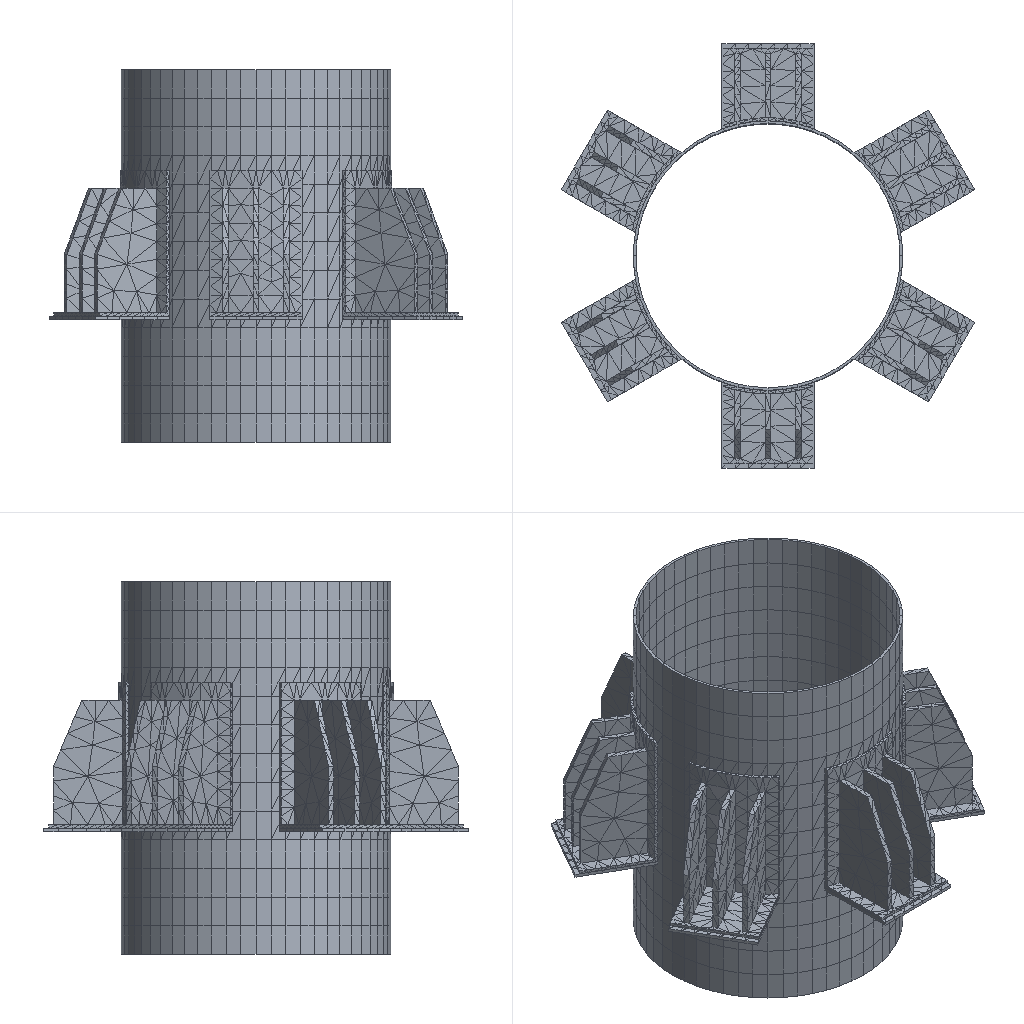Simulation study | ansys workbench
Ansys APDL input file, long lists of numbers shortened:
/batch
/config,noeldb,1     ! force off writing results to database
*get,_wallstrt,active,,time,wall
! ANSYS input file written by Workbench version 2022 R1
! File used for geometry attach:
/title,wbnew--____ (D5)
! ****** Begin Custom Load Command Snippet ******
/COM, ACT Extensions:
/COM,     LSDYNA, 2021.1
/COM,
! ****** End   Custom Load Command Snippet ******
*DIM,_wb_ProjectScratch_dir,string,248
_wb_ProjectScratch_dir(1) = ''
*DIM,_wb_SolverFiles_dir,string,248
_wb_SolverFiles_dir(1) = ''
*DIM,_wb_userfiles_dir,string,248
_wb_userfiles_dir(1) = ''
/com,--- Data in consistent NMM units. See Solving Units in the help system for more information.
/units,MPA
/nopr
/wb,file,start              !  signify a WB generated input file
/prep7
! Turn off shape checking because checks already performed inside WB mesher.
! See help system for more information.
SHPP,OFF,,NOWARN
/nolist
etcon,set             ! allow ANSYS to choose best KEYOP's for 180x elements, resets any applicable keyopt to MAPDL defaults
/com,*********** Nodes for the whole assembly ***********
nblock,3,,22077
(1i9,3e20.9e3)
        1     6.530950049E+02     2.499215719E+03     8.316464507E+02
! (20069 more lines like these left out)
-1
/wb,elem,start            !  set before creation of elements
/com,*********** Elements for Body 1 "__4^1400-589-450|__-__2" ***********
et,1,187
eblock,19,solid,,932
(19i9)
        1        1        1        1        0        0        0        0       10        0      729     5581     5723     5720     5722     7087     7383     7085     7086
! (1863 more lines like these left out)
-1
/com,*********** Elements for Body 2 "__5^1400-589-450|__-__1" ***********
et,2,186
keyo,2,2,1          ! set full integration on SOLID186
eblock,19,solid,,42
(19i9)
        2        2        2        2        0        0        0        0       20        0     6489    19376    19433    19434    19458    19377    19426    19425    19407
! (83 more lines like these left out)
-1
/com,*********** Elements for Body 3 "__5^1400-589-450|__-__1[2]" ***********
et,3,186
keyo,3,2,1          ! set full integration on SOLID186
eblock,19,solid,,42
(19i9)
        3        3        3        3        0        0        0        0       20        0     6405    18652    18709    18710    18734    18653    18702    18701    18683
! (83 more lines like these left out)
-1
/com,*********** Elements for Body 4 "__5^1400-589-450|__-__1[3]" ***********
et,4,186
keyo,4,2,1          ! set full integration on SOLID186
eblock,19,solid,,42
(19i9)
        4        4        4        4        0        0        0        0       20        0     6447    19014    19071    19072    19096    19015    19064    19063    19045
! (83 more lines like these left out)
-1
/com,*********** Elements for Body 5 "__5^1400-589-450|__-__1[4]" ***********
et,5,186
keyo,5,2,1          ! set full integration on SOLID186
eblock,19,solid,,42
(19i9)
        5        5        5        5        0        0        0        0       20        0     6531    19738    19795    19796    19820    19739    19788    19787    19769
! (83 more lines like these left out)
-1
/com,*********** Elements for Body 6 "__5^1400-589-450|__-__1[5]" ***********
et,6,186
keyo,6,2,1          ! set full integration on SOLID186
eblock,19,solid,,42
(19i9)
        6        6        6        6        0        0        0        0       20        0     6321    17928    17985    17986    18010    17929    17978    17977    17959
! (83 more lines like these left out)
-1
/com,*********** Elements for Body 7 "__5^1400-589-450|__-__1[6]" ***********
et,7,186
keyo,7,2,1          ! set full integration on SOLID186
eblock,19,solid,,42
(19i9)
        7        7        7        7        0        0        0        0       20        0     6363    18290    18347    18348    18372    18291    18340    18339    18321
! (83 more lines like these left out)
-1
/com,*********** Elements for Body 8 "__4^1400-589-450|__-__2[2]" ***********
et,8,187
eblock,19,solid,,932
(19i9)
        8        8        8        8        0        0        0        0       10        0     4457    13929    14071    14068    14070    15435    15731    15433    15434
! (1863 more lines like these left out)
-1
/com,*********** Elements for Body 9 "__4^1400-589-450|__-__2[3]" ***********
et,9,187
eblock,19,solid,,932
(19i9)
        9        9        9        9        0        0        0        0       10        0     3525    11842    11984    11981    11983    13348    13644    13346    13347
! (1863 more lines like these left out)
-1
/com,*********** Elements for Body 10 "__4^1400-589-450|__-__2[4]" ***********
et,10,187
eblock,19,solid,,932
(19i9)
       10       10       10       10        0        0        0        0       10        0     1661     7668     7810     7807     7809     9174     9470     9172     9173
! (1863 more lines like these left out)
-1
/com,*********** Elements for Body 11 "__4^1400-589-450|__-__2[5]" ***********
et,11,187
eblock,19,solid,,932
(19i9)
       11       11       11       11        0        0        0        0       10        0     5389    16016    16158    16155    16157    17522    17818    17520    17521
! (1863 more lines like these left out)
-1
/com,*********** Elements for Body 12 "__4^1400-589-450|__-__2[6]" ***********
et,12,187
eblock,19,solid,,932
(19i9)
       12       12       12       12        0        0        0        0       10        0     2593     9755     9897     9894     9896    11261    11557    11259    11260
! (1863 more lines like these left out)
-1
/com,*********** Elements for Body 13 "__3^1400-589-450|__-__1" ***********
et,13,186
keyo,13,2,1          ! set full integration on SOLID186
eblock,19,solid,,728
(19i9)
       13       13       13       13        0        0        0        0       20        0        1      113      893      843      478      437     1191      842      438
! (1455 more lines like these left out)
-1
/wb,elem,end               !  done creating elements
/com,*********** Send User Defined Coordinate System(s) ***********
csys,0
toffst,273.15,  ! Temperature offset from absolute zero
/com,*********** Set Reference Temperature ***********
tref,22.
/wb,mat,start              !  starting to send materials
/com,*********** Send Materials ***********
Temperature = 'TEMP' ! Temperature
MP,DENS,1,7.85e-09,	! tonne mm^-3
MP,ALPX,1,1.2e-05,	! C^-1
MP,C,1,434000000,	! mm^2 s^-2 C^-1
MP,KXX,1,60.5,	! tonne mm s^-3 C^-1
MP,RSVX,1,0.00017,	! ohm mm
MP,EX,1,200000,	! tonne s^-2 mm^-1
MP,NUXY,1,0.3,
MP,MURX,1,10000,
Temperature = 'TEMP' ! Temperature
MP,DENS,2,7.85e-09,	! tonne mm^-3
MP,ALPX,2,1.2e-05,	! C^-1
MP,C,2,434000000,	! mm^2 s^-2 C^-1
MP,KXX,2,60.5,	! tonne mm s^-3 C^-1
MP,RSVX,2,0.00017,	! ohm mm
MP,EX,2,200000,	! tonne s^-2 mm^-1
MP,NUXY,2,0.3,
MP,MURX,2,10000,
Temperature = 'TEMP' ! Temperature
MP,DENS,3,7.85e-09,	! tonne mm^-3
MP,ALPX,3,1.2e-05,	! C^-1
MP,C,3,434000000,	! mm^2 s^-2 C^-1
MP,KXX,3,60.5,	! tonne mm s^-3 C^-1
MP,RSVX,3,0.00017,	! ohm mm
MP,EX,3,200000,	! tonne s^-2 mm^-1
MP,NUXY,3,0.3,
MP,MURX,3,10000,
Temperature = 'TEMP' ! Temperature
MP,DENS,4,7.85e-09,	! tonne mm^-3
MP,ALPX,4,1.2e-05,	! C^-1
MP,C,4,434000000,	! mm^2 s^-2 C^-1
MP,KXX,4,60.5,	! tonne mm s^-3 C^-1
MP,RSVX,4,0.00017,	! ohm mm
MP,EX,4,200000,	! tonne s^-2 mm^-1
MP,NUXY,4,0.3,
MP,MURX,4,10000,
Temperature = 'TEMP' ! Temperature
MP,DENS,5,7.85e-09,	! tonne mm^-3
MP,ALPX,5,1.2e-05,	! C^-1
MP,C,5,434000000,	! mm^2 s^-2 C^-1
MP,KXX,5,60.5,	! tonne mm s^-3 C^-1
MP,RSVX,5,0.00017,	! ohm mm
MP,EX,5,200000,	! tonne s^-2 mm^-1
MP,NUXY,5,0.3,
MP,MURX,5,10000,
Temperature = 'TEMP' ! Temperature
MP,DENS,6,7.85e-09,	! tonne mm^-3
MP,ALPX,6,1.2e-05,	! C^-1
MP,C,6,434000000,	! mm^2 s^-2 C^-1
MP,KXX,6,60.5,	! tonne mm s^-3 C^-1
MP,RSVX,6,0.00017,	! ohm mm
MP,EX,6,200000,	! tonne s^-2 mm^-1
MP,NUXY,6,0.3,
MP,MURX,6,10000,
Temperature = 'TEMP' ! Temperature
MP,DENS,7,7.85e-09,	! tonne mm^-3
MP,ALPX,7,1.2e-05,	! C^-1
MP,C,7,434000000,	! mm^2 s^-2 C^-1
MP,KXX,7,60.5,	! tonne mm s^-3 C^-1
MP,RSVX,7,0.00017,	! ohm mm
MP,EX,7,200000,	! tonne s^-2 mm^-1
MP,NUXY,7,0.3,
MP,MURX,7,10000,
Temperature = 'TEMP' ! Temperature
MP,DENS,8,7.85e-09,	! tonne mm^-3
MP,ALPX,8,1.2e-05,	! C^-1
MP,C,8,434000000,	! mm^2 s^-2 C^-1
MP,KXX,8,60.5,	! tonne mm s^-3 C^-1
MP,RSVX,8,0.00017,	! ohm mm
MP,EX,8,200000,	! tonne s^-2 mm^-1
MP,NUXY,8,0.3,
MP,MURX,8,10000,
Temperature = 'TEMP' ! Temperature
MP,DENS,9,7.85e-09,	! tonne mm^-3
MP,ALPX,9,1.2e-05,	! C^-1
MP,C,9,434000000,	! mm^2 s^-2 C^-1
MP,KXX,9,60.5,	! tonne mm s^-3 C^-1
MP,RSVX,9,0.00017,	! ohm mm
MP,EX,9,200000,	! tonne s^-2 mm^-1
MP,NUXY,9,0.3,
MP,MURX,9,10000,
Temperature = 'TEMP' ! Temperature
MP,DENS,10,7.85e-09,	! tonne mm^-3
MP,ALPX,10,1.2e-05,	! C^-1
MP,C,10,434000000,	! mm^2 s^-2 C^-1
MP,KXX,10,60.5,	! tonne mm s^-3 C^-1
MP,RSVX,10,0.00017,	! ohm mm
MP,EX,10,200000,	! tonne s^-2 mm^-1
MP,NUXY,10,0.3,
MP,MURX,10,10000,
Temperature = 'TEMP' ! Temperature
MP,DENS,11,7.85e-09,	! tonne mm^-3
MP,ALPX,11,1.2e-05,	! C^-1
MP,C,11,434000000,	! mm^2 s^-2 C^-1
MP,KXX,11,60.5,	! tonne mm s^-3 C^-1
MP,RSVX,11,0.00017,	! ohm mm
MP,EX,11,200000,	! tonne s^-2 mm^-1
MP,NUXY,11,0.3,
MP,MURX,11,10000,
Temperature = 'TEMP' ! Temperature
MP,DENS,12,7.85e-09,	! tonne mm^-3
MP,ALPX,12,1.2e-05,	! C^-1
MP,C,12,434000000,	! mm^2 s^-2 C^-1
MP,KXX,12,60.5,	! tonne mm s^-3 C^-1
MP,RSVX,12,0.00017,	! ohm mm
MP,EX,12,200000,	! tonne s^-2 mm^-1
MP,NUXY,12,0.3,
MP,MURX,12,10000,
Temperature = 'TEMP' ! Temperature
MP,DENS,13,7.85e-09,	! tonne mm^-3
MP,ALPX,13,1.2e-05,	! C^-1
MP,C,13,434000000,	! mm^2 s^-2 C^-1
MP,KXX,13,60.5,	! tonne mm s^-3 C^-1
MP,RSVX,13,0.00017,	! ohm mm
MP,EX,13,200000,	! tonne s^-2 mm^-1
MP,NUXY,13,0.3,
MP,MURX,13,10000,
/wb,mat,end                !  done sending materials
!************************* Model Summary ********************
!__4^1400-589-450|__-__2,	Q345B,	matid,	1
!__5^1400-589-450|__-__1,	Q345B,	matid,	2
!__5^1400-589-450|__-__1[2],	Q345B,	matid,	3
!__5^1400-589-450|__-__1[3],	Q345B,	matid,	4
!__5^1400-589-450|__-__1[4],	Q345B,	matid,	5
!__5^1400-589-450|__-__1[5],	Q345B,	matid,	6
!__5^1400-589-450|__-__1[6],	Q345B,	matid,	7
!__4^1400-589-450|__-__2[2],	Q345B,	matid,	8
!__4^1400-589-450|__-__2[3],	Q345B,	matid,	9
!__4^1400-589-450|__-__2[4],	Q345B,	matid,	10
!__4^1400-589-450|__-__2[5],	Q345B,	matid,	11
!__4^1400-589-450|__-__2[6],	Q345B,	matid,	12
!__3^1400-589-450|__-__1,	Q345B,	matid,	13
!************************* End Model Summary ********************
! get the diagonal of the bounding box. Needed later for other things
*get,_xmin,node,,mnloc,x
*get,_ymin,node,,mnloc,y
*get,_zmin,node,,mnloc,z
*get,_xmax,node,,mxloc,x
*get,_ymax,node,,mxloc,y
*get,_zmax,node,,mxloc,z
_ASMDIAG=(_xmax-_xmin)*(_xmax-_xmin)+(_ymax-_ymin)*(_ymax-_ymin)+(_zmax-_zmin)*(_zmax-_zmin)
_ASMDIAG=SQRT(_ASMDIAG)
/wb,contact,start          !  starting to send contact
/com,*********** Create Contact "接触区域" ***********
/com,            Real Constant Set For Above Contact Is 15 & 14
*set,tid,15
*set,cid,14
r,tid
r,cid
et,tid,170
et,cid,174
eblock,10,,,72
(15i9)
    13409       15       15       15        0     5471     5650     5491     5491     6483     6587     5491     6480
! (71 more lines like these left out)
-1
eblock,10,,,72
(15i9)
    13481       14       14       14        0     5471     5650     5491     5491     6483     6587     5491     6480
! (71 more lines like these left out)
-1
eblock,10,,,42
(15i9)
    13553       14       15       14        0    19407    19377    19426    19425    19562    19563    19668    19632
! (41 more lines like these left out)
-1
eblock,10,,,42
(15i9)
    13595       15       14       15        0    19407    19377    19426    19425    19562    19563    19668    19632
! (41 more lines like these left out)
-1
keyo,cid,8,2               ! auto create asymmetric contact (from Program Controlled setting)
keyo,cid,10,0              ! adjust contact stiffness each NR iteration (from Program Controlled setting)
keyo,cid,12,5              ! bonded always
keyo,cid,18,1              ! small sliding turned on by application
keyo,cid,2,0               ! augmented Lagrange (from Program Controlled setting)
keyo,cid,4,0               ! on Gauss point (from Program Controlled setting)
keyo,cid,9,1               ! ignore initial gaps/penetration
keyo,cid,7,0               ! No Prediction
rmod,tid,3,10.      ! FKN
rmod,tid,5,0.       ! ICONT
rmod,tid,6,0.       ! PINB
rmod,tid,10,0.      ! CNOF
rmod,tid,12,0.      ! FKT
rmod,tid,36,62      ! WB DSID
rmod,cid,3,10.      ! FKN
rmod,cid,5,0.       ! ICONT
rmod,cid,6,0.       ! PINB
rmod,cid,10,0.      ! CNOF
rmod,cid,12,0.      ! FKT
rmod,cid,36,62      ! WB DSID
/com,*********** Create Contact "接触区域 2" ***********
/com,            Real Constant Set For Above Contact Is 17 & 16
*set,tid,17
*set,cid,16
r,tid
r,cid
et,tid,170
et,cid,174
eblock,10,,,124
(15i9)
    13637       17       17       17        0     5616     5452     5683     5683     6386     6388     5683     7179
! (123 more lines like these left out)
-1
eblock,10,,,124
(15i9)
    13761       16       16       16        0     5616     5452     5683     5683     6386     6388     5683     7179
! (123 more lines like these left out)
-1
eblock,10,,,48
(15i9)
    13885       16       17       16        0      984      985      958      957     4310     4260     4257     4258
! (47 more lines like these left out)
-1
eblock,10,,,48
(15i9)
    13933       17       16       17        0      984      985      958      957     4310     4260     4257     4258
! (47 more lines like these left out)
-1
keyo,cid,8,2               ! auto create asymmetric contact (from Program Controlled setting)
keyo,cid,10,0              ! adjust contact stiffness each NR iteration (from Program Controlled setting)
keyo,cid,12,5              ! bonded always
keyo,cid,18,1              ! small sliding turned on by application
keyo,cid,2,0               ! augmented Lagrange (from Program Controlled setting)
keyo,cid,4,0               ! on Gauss point (from Program Controlled setting)
keyo,cid,9,1               ! ignore initial gaps/penetration
keyo,cid,7,0               ! No Prediction
rmod,tid,3,10.      ! FKN
rmod,tid,5,0.       ! ICONT
rmod,tid,6,0.       ! PINB
rmod,tid,10,0.      ! CNOF
rmod,tid,12,0.      ! FKT
rmod,tid,36,65      ! WB DSID
rmod,cid,3,10.      ! FKN
rmod,cid,5,0.       ! ICONT
rmod,cid,6,0.       ! PINB
rmod,cid,10,0.      ! CNOF
rmod,cid,12,0.      ! FKT
rmod,cid,36,65      ! WB DSID
/com,*********** Create Contact "接触区域 3" ***********
/com,            Real Constant Set For Above Contact Is 19 & 18
*set,tid,19
*set,cid,18
r,tid
r,cid
et,tid,170
et,cid,174
eblock,10,,,7
(15i9)
    13981       19       19       19        0    19440    19439    19432    19431    19690    19682    19680    19681
! (6 more lines like these left out)
-1
eblock,10,,,7
(15i9)
    13988       18       18       18        0    19440    19439    19432    19431    19690    19682    19680    19681
! (6 more lines like these left out)
-1
eblock,10,,,8
(15i9)
    13995       18       19       18        0      984      985      958      957     4310     4260     4257     4258
! (7 more lines like these left out)
-1
eblock,10,,,8
(15i9)
    14003       19       18       19        0      984      985      958      957     4310     4260     4257     4258
! (7 more lines like these left out)
-1
keyo,cid,8,2               ! auto create asymmetric contact (from Program Controlled setting)
keyo,cid,10,0              ! adjust contact stiffness each NR iteration (from Program Controlled setting)
keyo,cid,12,5              ! bonded always
keyo,cid,18,1              ! small sliding turned on by application
keyo,cid,2,0               ! augmented Lagrange (from Program Controlled setting)
keyo,cid,4,0               ! on Gauss point (from Program Controlled setting)
keyo,cid,9,1               ! ignore initial gaps/penetration
keyo,cid,7,0               ! No Prediction
rmod,tid,3,10.      ! FKN
rmod,tid,5,0.       ! ICONT
rmod,tid,6,0.       ! PINB
rmod,tid,10,0.      ! CNOF
rmod,tid,12,0.      ! FKT
rmod,tid,36,68      ! WB DSID
rmod,cid,3,10.      ! FKN
rmod,cid,5,0.       ! ICONT
rmod,cid,6,0.       ! PINB
rmod,cid,10,0.      ! CNOF
rmod,cid,12,0.      ! FKT
rmod,cid,36,68      ! WB DSID
/com,*********** Create Contact "接触区域 4" ***********
/com,            Real Constant Set For Above Contact Is 21 & 20
*set,tid,21
*set,cid,20
r,tid
r,cid
et,tid,170
et,cid,174
eblock,10,,,42
(15i9)
    14011       21       21       21        0    18683    18653    18702    18701    18838    18839    18944    18908
! (41 more lines like these left out)
-1
eblock,10,,,42
(15i9)
    14053       20       20       20        0    18683    18653    18702    18701    18838    18839    18944    18908
! (41 more lines like these left out)
-1
eblock,10,,,72
(15i9)
    14095       20       21       20        0    13819    13998    13839    13839    14831    14935    13839    14828
! (71 more lines like these left out)
-1
eblock,10,,,72
(15i9)
    14167       21       20       21        0    13819    13998    13839    13839    14831    14935    13839    14828
! (71 more lines like these left out)
-1
keyo,cid,8,2               ! auto create asymmetric contact (from Program Controlled setting)
keyo,cid,10,0              ! adjust contact stiffness each NR iteration (from Program Controlled setting)
keyo,cid,12,5              ! bonded always
keyo,cid,18,1              ! small sliding turned on by application
keyo,cid,2,0               ! augmented Lagrange (from Program Controlled setting)
keyo,cid,4,0               ! on Gauss point (from Program Controlled setting)
keyo,cid,9,1               ! ignore initial gaps/penetration
keyo,cid,7,0               ! No Prediction
rmod,tid,3,10.      ! FKN
rmod,tid,5,0.       ! ICONT
rmod,tid,6,0.       ! PINB
rmod,tid,10,0.      ! CNOF
rmod,tid,12,0.      ! FKT
rmod,tid,36,71      ! WB DSID
rmod,cid,3,10.      ! FKN
rmod,cid,5,0.       ! ICONT
rmod,cid,6,0.       ! PINB
rmod,cid,10,0.      ! CNOF
rmod,cid,12,0.      ! FKT
rmod,cid,36,71      ! WB DSID
/com,*********** Create Contact "接触区域 5" ***********
/com,            Real Constant Set For Above Contact Is 23 & 22
*set,tid,23
*set,cid,22
r,tid
r,cid
et,tid,170
et,cid,174
eblock,10,,,7
(15i9)
    14239       23       23       23        0    18716    18715    18708    18707    18966    18958    18956    18957
! (6 more lines like these left out)
-1
eblock,10,,,7
(15i9)
    14246       22       22       22        0    18716    18715    18708    18707    18966    18958    18956    18957
! (6 more lines like these left out)
-1
eblock,10,,,8
(15i9)
    14253       22       23       22        0      975      976      949      948     4292     4242     4239     4240
! (7 more lines like these left out)
-1
eblock,10,,,8
(15i9)
    14261       23       22       23        0      975      976      949      948     4292     4242     4239     4240
! (7 more lines like these left out)
-1
keyo,cid,8,2               ! auto create asymmetric contact (from Program Controlled setting)
keyo,cid,10,0              ! adjust contact stiffness each NR iteration (from Program Controlled setting)
keyo,cid,12,5              ! bonded always
keyo,cid,18,1              ! small sliding turned on by application
keyo,cid,2,0               ! augmented Lagrange (from Program Controlled setting)
keyo,cid,4,0               ! on Gauss point (from Program Controlled setting)
keyo,cid,9,1               ! ignore initial gaps/penetration
keyo,cid,7,0               ! No Prediction
rmod,tid,3,10.      ! FKN
rmod,tid,5,0.       ! ICONT
rmod,tid,6,0.       ! PINB
rmod,tid,10,0.      ! CNOF
rmod,tid,12,0.      ! FKT
rmod,tid,36,74      ! WB DSID
rmod,cid,3,10.      ! FKN
rmod,cid,5,0.       ! ICONT
rmod,cid,6,0.       ! PINB
rmod,cid,10,0.      ! CNOF
rmod,cid,12,0.      ! FKT
rmod,cid,36,74      ! WB DSID
/com,*********** Create Contact "接触区域 6" ***********
/com,            Real Constant Set For Above Contact Is 25 & 24
*set,tid,25
*set,cid,24
r,tid
r,cid
et,tid,170
et,cid,174
eblock,10,,,42
(15i9)
    14269       25       25       25        0    19045    19015    19064    19063    19200    19201    19306    19270
! (41 more lines like these left out)
-1
eblock,10,,,42
(15i9)
    14311       24       24       24        0    19045    19015    19064    19063    19200    19201    19306    19270
! (41 more lines like these left out)
-1
eblock,10,,,72
(15i9)
    14353       24       25       24        0    11732    11911    11752    11752    12744    12848    11752    12741
! (71 more lines like these left out)
-1
eblock,10,,,72
(15i9)
    14425       25       24       25        0    11732    11911    11752    11752    12744    12848    11752    12741
! (71 more lines like these left out)
-1
keyo,cid,8,2               ! auto create asymmetric contact (from Program Controlled setting)
keyo,cid,10,0              ! adjust contact stiffness each NR iteration (from Program Controlled setting)
keyo,cid,12,5              ! bonded always
keyo,cid,18,1              ! small sliding turned on by application
keyo,cid,2,0               ! augmented Lagrange (from Program Controlled setting)
keyo,cid,4,0               ! on Gauss point (from Program Controlled setting)
keyo,cid,9,1               ! ignore initial gaps/penetration
keyo,cid,7,0               ! No Prediction
rmod,tid,3,10.      ! FKN
rmod,tid,5,0.       ! ICONT
rmod,tid,6,0.       ! PINB
rmod,tid,10,0.      ! CNOF
rmod,tid,12,0.      ! FKT
rmod,tid,36,77      ! WB DSID
rmod,cid,3,10.      ! FKN
rmod,cid,5,0.       ! ICONT
rmod,cid,6,0.       ! PINB
rmod,cid,10,0.      ! CNOF
rmod,cid,12,0.      ! FKT
rmod,cid,36,77      ! WB DSID
/com,*********** Create Contact "接触区域 7" ***********
/com,            Real Constant Set For Above Contact Is 27 & 26
*set,tid,27
*set,cid,26
r,tid
r,cid
et,tid,170
et,cid,174
eblock,10,,,7
(15i9)
    14497       27       27       27        0    19078    19077    19070    19069    19328    19320    19318    19319
! (6 more lines like these left out)
-1
eblock,10,,,7
(15i9)
    14504       26       26       26        0    19078    19077    19070    19069    19328    19320    19318    19319
! (6 more lines like these left out)
-1
eblock,10,,,8
(15i9)
    14511       26       27       26        0      616      617      590      589     3374     3296     3292     3293
! (7 more lines like these left out)
-1
eblock,10,,,8
(15i9)
    14519       27       26       27        0      616      617      590      589     3374     3296     3292     3293
! (7 more lines like these left out)
-1
keyo,cid,8,2               ! auto create asymmetric contact (from Program Controlled setting)
keyo,cid,10,0              ! adjust contact stiffness each NR iteration (from Program Controlled setting)
keyo,cid,12,5              ! bonded always
keyo,cid,18,1              ! small sliding turned on by application
keyo,cid,2,0               ! augmented Lagrange (from Program Controlled setting)
keyo,cid,4,0               ! on Gauss point (from Program Controlled setting)
keyo,cid,9,1               ! ignore initial gaps/penetration
keyo,cid,7,0               ! No Prediction
rmod,tid,3,10.      ! FKN
rmod,tid,5,0.       ! ICONT
rmod,tid,6,0.       ! PINB
rmod,tid,10,0.      ! CNOF
rmod,tid,12,0.      ! FKT
rmod,tid,36,80      ! WB DSID
rmod,cid,3,10.      ! FKN
rmod,cid,5,0.       ! ICONT
rmod,cid,6,0.       ! PINB
rmod,cid,10,0.      ! CNOF
rmod,cid,12,0.      ! FKT
rmod,cid,36,80      ! WB DSID
/com,*********** Create Contact "接触区域 8" ***********
/com,            Real Constant Set For Above Contact Is 29 & 28
*set,tid,29
*set,cid,28
r,tid
r,cid
et,tid,170
et,cid,174
eblock,10,,,42
(15i9)
    14527       29       29       29        0    19769    19739    19788    19787    19924    19925    20030    19994
! (41 more lines like these left out)
-1
eblock,10,,,42
(15i9)
    14569       28       28       28        0    19769    19739    19788    19787    19924    19925    20030    19994
! (41 more lines like these left out)
-1
eblock,10,,,72
(15i9)
    14611       28       29       28        0     7558     7737     7578     7578     8570     8674     7578     8567
! (71 more lines like these left out)
-1
eblock,10,,,72
(15i9)
    14683       29       28       29        0     7558     7737     7578     7578     8570     8674     7578     8567
! (71 more lines like these left out)
-1
keyo,cid,8,2               ! auto create asymmetric contact (from Program Controlled setting)
keyo,cid,10,0              ! adjust contact stiffness each NR iteration (from Program Controlled setting)
keyo,cid,12,5              ! bonded always
keyo,cid,18,1              ! small sliding turned on by application
keyo,cid,2,0               ! augmented Lagrange (from Program Controlled setting)
keyo,cid,4,0               ! on Gauss point (from Program Controlled setting)
keyo,cid,9,1               ! ignore initial gaps/penetration
keyo,cid,7,0               ! No Prediction
rmod,tid,3,10.      ! FKN
rmod,tid,5,0.       ! ICONT
rmod,tid,6,0.       ! PINB
rmod,tid,10,0.      ! CNOF
rmod,tid,12,0.      ! FKT
rmod,tid,36,83      ! WB DSID
rmod,cid,3,10.      ! FKN
rmod,cid,5,0.       ! ICONT
rmod,cid,6,0.       ! PINB
rmod,cid,10,0.      ! CNOF
rmod,cid,12,0.      ! FKT
rmod,cid,36,83      ! WB DSID
/com,*********** Create Contact "接触区域 9" ***********
/com,            Real Constant Set For Above Contact Is 31 & 30
*set,tid,31
*set,cid,30
r,tid
r,cid
et,tid,170
et,cid,174
eblock,10,,,7
(15i9)
    14755       31       31       31        0    19802    19801    19794    19793    20052    20044    20042    20043
! (6 more lines like these left out)
-1
eblock,10,,,7
(15i9)
    14762       30       30       30        0    19802    19801    19794    19793    20052    20044    20042    20043
! (6 more lines like these left out)
-1
eblock,10,,,8
(15i9)
    14769       30       31       30        0      607      608      581      580     3347     3269     3265     3266
! (7 more lines like these left out)
-1
eblock,10,,,8
(15i9)
    14777       31       30       31        0      607      608      581      580     3347     3269     3265     3266
! (7 more lines like these left out)
-1
keyo,cid,8,2               ! auto create asymmetric contact (from Program Controlled setting)
keyo,cid,10,0              ! adjust contact stiffness each NR iteration (from Program Controlled setting)
keyo,cid,12,5              ! bonded always
keyo,cid,18,1              ! small sliding turned on by application
keyo,cid,2,0               ! augmented Lagrange (from Program Controlled setting)
keyo,cid,4,0               ! on Gauss point (from Program Controlled setting)
keyo,cid,9,1               ! ignore initial gaps/penetration
keyo,cid,7,0               ! No Prediction
rmod,tid,3,10.      ! FKN
rmod,tid,5,0.       ! ICONT
rmod,tid,6,0.       ! PINB
rmod,tid,10,0.      ! CNOF
rmod,tid,12,0.      ! FKT
rmod,tid,36,86      ! WB DSID
rmod,cid,3,10.      ! FKN
rmod,cid,5,0.       ! ICONT
rmod,cid,6,0.       ! PINB
rmod,cid,10,0.      ! CNOF
rmod,cid,12,0.      ! FKT
rmod,cid,36,86      ! WB DSID
/com,*********** Create Contact "接触区域 10" ***********
/com,            Real Constant Set For Above Contact Is 33 & 32
*set,tid,33
*set,cid,32
r,tid
r,cid
et,tid,170
et,cid,174
eblock,10,,,42
(15i9)
    14785       33       33       33        0    17959    17929    17978    17977    18114    18115    18220    18184
! (41 more lines like these left out)
-1
eblock,10,,,42
(15i9)
    14827       32       32       32        0    17959    17929    17978    17977    18114    18115    18220    18184
! (41 more lines like these left out)
-1
eblock,10,,,72
(15i9)
    14869       32       33       32        0    15906    16085    15926    15926    16918    17022    15926    16915
! (71 more lines like these left out)
-1
eblock,10,,,72
(15i9)
    14941       33       32       33        0    15906    16085    15926    15926    16918    17022    15926    16915
! (71 more lines like these left out)
-1
keyo,cid,8,2               ! auto create asymmetric contact (from Program Controlled setting)
keyo,cid,10,0              ! adjust contact stiffness each NR iteration (from Program Controlled setting)
keyo,cid,12,5              ! bonded always
keyo,cid,18,1              ! small sliding turned on by application
keyo,cid,2,0               ! augmented Lagrange (from Program Controlled setting)
keyo,cid,4,0               ! on Gauss point (from Program Controlled setting)
keyo,cid,9,1               ! ignore initial gaps/penetration
keyo,cid,7,0               ! No Prediction
rmod,tid,3,10.      ! FKN
rmod,tid,5,0.       ! ICONT
rmod,tid,6,0.       ! PINB
rmod,tid,10,0.      ! CNOF
rmod,tid,12,0.      ! FKT
rmod,tid,36,89      ! WB DSID
rmod,cid,3,10.      ! FKN
rmod,cid,5,0.       ! ICONT
rmod,cid,6,0.       ! PINB
rmod,cid,10,0.      ! CNOF
rmod,cid,12,0.      ! FKT
rmod,cid,36,89      ! WB DSID
/com,*********** Create Contact "接触区域 11" ***********
/com,            Real Constant Set For Above Contact Is 35 & 34
*set,tid,35
*set,cid,34
r,tid
r,cid
et,tid,170
et,cid,174
eblock,10,,,7
(15i9)
    15013       35       35       35        0    17992    17991    17984    17983    18242    18234    18232    18233
! (6 more lines like these left out)
-1
eblock,10,,,7
(15i9)
    15020       34       34       34        0    17992    17991    17984    17983    18242    18234    18232    18233
! (6 more lines like these left out)
-1
eblock,10,,,8
(15i9)
    15027       34       35       34        0      598      599      572      571     3319     3242     3237     3238
! (7 more lines like these left out)
-1
eblock,10,,,8
(15i9)
    15035       35       34       35        0      598      599      572      571     3319     3242     3237     3238
! (7 more lines like these left out)
-1
keyo,cid,8,2               ! auto create asymmetric contact (from Program Controlled setting)
keyo,cid,10,0              ! adjust contact stiffness each NR iteration (from Program Controlled setting)
keyo,cid,12,5              ! bonded always
keyo,cid,18,1              ! small sliding turned on by application
keyo,cid,2,0               ! augmented Lagrange (from Program Controlled setting)
keyo,cid,4,0               ! on Gauss point (from Program Controlled setting)
keyo,cid,9,1               ! ignore initial gaps/penetration
keyo,cid,7,0               ! No Prediction
rmod,tid,3,10.      ! FKN
rmod,tid,5,0.       ! ICONT
rmod,tid,6,0.       ! PINB
rmod,tid,10,0.      ! CNOF
rmod,tid,12,0.      ! FKT
rmod,tid,36,92      ! WB DSID
rmod,cid,3,10.      ! FKN
rmod,cid,5,0.       ! ICONT
rmod,cid,6,0.       ! PINB
rmod,cid,10,0.      ! CNOF
rmod,cid,12,0.      ! FKT
rmod,cid,36,92      ! WB DSID
/com,*********** Create Contact "接触区域 12" ***********
/com,            Real Constant Set For Above Contact Is 37 & 36
*set,tid,37
*set,cid,36
r,tid
r,cid
et,tid,170
et,cid,174
eblock,10,,,42
(15i9)
    15043       37       37       37        0    18321    18291    18340    18339    18476    18477    18582    18546
! (41 more lines like these left out)
-1
eblock,10,,,42
(15i9)
    15085       36       36       36        0    18321    18291    18340    18339    18476    18477    18582    18546
! (41 more lines like these left out)
-1
eblock,10,,,72
(15i9)
    15127       36       37       36        0     9645     9824     9665     9665    10657    10761     9665    10654
! (71 more lines like these left out)
-1
eblock,10,,,72
(15i9)
    15199       37       36       37        0     9645     9824     9665     9665    10657    10761     9665    10654
! (71 more lines like these left out)
-1
keyo,cid,8,2               ! auto create asymmetric contact (from Program Controlled setting)
keyo,cid,10,0              ! adjust contact stiffness each NR iteration (from Program Controlled setting)
keyo,cid,12,5              ! bonded always
keyo,cid,18,1              ! small sliding turned on by application
keyo,cid,2,0               ! augmented Lagrange (from Program Controlled setting)
keyo,cid,4,0               ! on Gauss point (from Program Controlled setting)
keyo,cid,9,1               ! ignore initial gaps/penetration
keyo,cid,7,0               ! No Prediction
rmod,tid,3,10.      ! FKN
rmod,tid,5,0.       ! ICONT
rmod,tid,6,0.       ! PINB
rmod,tid,10,0.      ! CNOF
rmod,tid,12,0.      ! FKT
rmod,tid,36,95      ! WB DSID
rmod,cid,3,10.      ! FKN
rmod,cid,5,0.       ! ICONT
rmod,cid,6,0.       ! PINB
rmod,cid,10,0.      ! CNOF
rmod,cid,12,0.      ! FKT
rmod,cid,36,95      ! WB DSID
/com,*********** Create Contact "接触区域 13" ***********
/com,            Real Constant Set For Above Contact Is 39 & 38
*set,tid,39
*set,cid,38
r,tid
r,cid
et,tid,170
et,cid,174
eblock,10,,,7
(15i9)
    15271       39       39       39        0    18354    18353    18346    18345    18604    18596    18594    18595
! (6 more lines like these left out)
-1
eblock,10,,,7
(15i9)
    15278       38       38       38        0    18354    18353    18346    18345    18604    18596    18594    18595
! (6 more lines like these left out)
-1
eblock,10,,,8
(15i9)
    15285       38       39       38        0      993      994      967      966     4328     4278     4275     4276
! (7 more lines like these left out)
-1
eblock,10,,,8
(15i9)
    15293       39       38       39        0      993      994      967      966     4328     4278     4275     4276
! (7 more lines like these left out)
-1
keyo,cid,8,2               ! auto create asymmetric contact (from Program Controlled setting)
keyo,cid,10,0              ! adjust contact stiffness each NR iteration (from Program Controlled setting)
keyo,cid,12,5              ! bonded always
keyo,cid,18,1              ! small sliding turned on by application
keyo,cid,2,0               ! augmented Lagrange (from Program Controlled setting)
keyo,cid,4,0               ! on Gauss point (from Program Controlled setting)
keyo,cid,9,1               ! ignore initial gaps/penetration
keyo,cid,7,0               ! No Prediction
rmod,tid,3,10.      ! FKN
rmod,tid,5,0.       ! ICONT
rmod,tid,6,0.       ! PINB
rmod,tid,10,0.      ! CNOF
rmod,tid,12,0.      ! FKT
rmod,tid,36,98      ! WB DSID
rmod,cid,3,10.      ! FKN
rmod,cid,5,0.       ! ICONT
rmod,cid,6,0.       ! PINB
rmod,cid,10,0.      ! CNOF
rmod,cid,12,0.      ! FKT
rmod,cid,36,98      ! WB DSID
/com,*********** Create Contact "接触区域 14" ***********
/com,            Real Constant Set For Above Contact Is 41 & 40
*set,tid,41
*set,cid,40
r,tid
r,cid
et,tid,170
et,cid,174
eblock,10,,,124
(15i9)
    15301       41       41       41        0    13964    13800    14031    14031    14734    14736    14031    15527
! (123 more lines like these left out)
-1
eblock,10,,,124
(15i9)
    15425       40       40       40        0    13964    13800    14031    14031    14734    14736    14031    15527
! (123 more lines like these left out)
-1
eblock,10,,,48
(15i9)
    15549       40       41       40        0      975      976      949      948     4292     4242     4239     4240
! (47 more lines like these left out)
-1
eblock,10,,,48
(15i9)
    15597       41       40       41        0      975      976      949      948     4292     4242     4239     4240
! (47 more lines like these left out)
-1
keyo,cid,8,2               ! auto create asymmetric contact (from Program Controlled setting)
keyo,cid,10,0              ! adjust contact stiffness each NR iteration (from Program Controlled setting)
keyo,cid,12,5              ! bonded always
keyo,cid,18,1              ! small sliding turned on by application
keyo,cid,2,0               ! augmented Lagrange (from Program Controlled setting)
keyo,cid,4,0               ! on Gauss point (from Program Controlled setting)
keyo,cid,9,1               ! ignore initial gaps/penetration
keyo,cid,7,0               ! No Prediction
rmod,tid,3,10.      ! FKN
rmod,tid,5,0.       ! ICONT
rmod,tid,6,0.       ! PINB
rmod,tid,10,0.      ! CNOF
rmod,tid,12,0.      ! FKT
rmod,tid,36,101     ! WB DSID
rmod,cid,3,10.      ! FKN
rmod,cid,5,0.       ! ICONT
rmod,cid,6,0.       ! PINB
rmod,cid,10,0.      ! CNOF
rmod,cid,12,0.      ! FKT
rmod,cid,36,101     ! WB DSID
/com,*********** Create Contact "接触区域 15" ***********
/com,            Real Constant Set For Above Contact Is 43 & 42
*set,tid,43
*set,cid,42
r,tid
r,cid
et,tid,170
et,cid,174
eblock,10,,,124
(15i9)
    15645       43       43       43        0    11877    11713    11944    11944    12647    12649    11944    13440
! (123 more lines like these left out)
-1
eblock,10,,,124
(15i9)
    15769       42       42       42        0    11877    11713    11944    11944    12647    12649    11944    13440
! (123 more lines like these left out)
-1
eblock,10,,,48
(15i9)
    15893       42       43       42        0      616      617      590      589     3374     3296     3292     3293
! (47 more lines like these left out)
-1
eblock,10,,,48
(15i9)
    15941       43       42       43        0      616      617      590      589     3374     3296     3292     3293
! (47 more lines like these left out)
-1
keyo,cid,8,2               ! auto create asymmetric contact (from Program Controlled setting)
keyo,cid,10,0              ! adjust contact stiffness each NR iteration (from Program Controlled setting)
keyo,cid,12,5              ! bonded always
keyo,cid,18,1              ! small sliding turned on by application
keyo,cid,2,0               ! augmented Lagrange (from Program Controlled setting)
keyo,cid,4,0               ! on Gauss point (from Program Controlled setting)
keyo,cid,9,1               ! ignore initial gaps/penetration
keyo,cid,7,0               ! No Prediction
rmod,tid,3,10.      ! FKN
rmod,tid,5,0.       ! ICONT
rmod,tid,6,0.       ! PINB
rmod,tid,10,0.      ! CNOF
rmod,tid,12,0.      ! FKT
rmod,tid,36,104     ! WB DSID
rmod,cid,3,10.      ! FKN
rmod,cid,5,0.       ! ICONT
rmod,cid,6,0.       ! PINB
rmod,cid,10,0.      ! CNOF
rmod,cid,12,0.      ! FKT
rmod,cid,36,104     ! WB DSID
/com,*********** Create Contact "接触区域 16" ***********
/com,            Real Constant Set For Above Contact Is 45 & 44
*set,tid,45
*set,cid,44
r,tid
r,cid
et,tid,170
et,cid,174
eblock,10,,,124
(15i9)
    15989       45       45       45        0     7703     7539     7770     7770     8473     8475     7770     9266
! (123 more lines like these left out)
-1
eblock,10,,,124
(15i9)
    16113       44       44       44        0     7703     7539     7770     7770     8473     8475     7770     9266
! (123 more lines like these left out)
-1
eblock,10,,,48
(15i9)
    16237       44       45       44        0      607      608      581      580     3347     3269     3265     3266
! (47 more lines like these left out)
-1
eblock,10,,,48
(15i9)
    16285       45       44       45        0      607      608      581      580     3347     3269     3265     3266
! (47 more lines like these left out)
-1
keyo,cid,8,2               ! auto create asymmetric contact (from Program Controlled setting)
keyo,cid,10,0              ! adjust contact stiffness each NR iteration (from Program Controlled setting)
keyo,cid,12,5              ! bonded always
keyo,cid,18,1              ! small sliding turned on by application
keyo,cid,2,0               ! augmented Lagrange (from Program Controlled setting)
keyo,cid,4,0               ! on Gauss point (from Program Controlled setting)
keyo,cid,9,1               ! ignore initial gaps/penetration
keyo,cid,7,0               ! No Prediction
rmod,tid,3,10.      ! FKN
rmod,tid,5,0.       ! ICONT
rmod,tid,6,0.       ! PINB
rmod,tid,10,0.      ! CNOF
rmod,tid,12,0.      ! FKT
rmod,tid,36,107     ! WB DSID
rmod,cid,3,10.      ! FKN
rmod,cid,5,0.       ! ICONT
rmod,cid,6,0.       ! PINB
rmod,cid,10,0.      ! CNOF
rmod,cid,12,0.      ! FKT
rmod,cid,36,107     ! WB DSID
/com,*********** Create Contact "接触区域 17" ***********
/com,            Real Constant Set For Above Contact Is 47 & 46
*set,tid,47
*set,cid,46
r,tid
r,cid
et,tid,170
et,cid,174
eblock,10,,,124
(15i9)
    16333       47       47       47        0    16051    15887    16118    16118    16821    16823    16118    17614
! (123 more lines like these left out)
-1
eblock,10,,,124
(15i9)
    16457       46       46       46        0    16051    15887    16118    16118    16821    16823    16118    17614
! (123 more lines like these left out)
-1
eblock,10,,,48
(15i9)
    16581       46       47       46        0      598      599      572      571     3319     3242     3237     3238
! (47 more lines like these left out)
-1
eblock,10,,,48
(15i9)
    16629       47       46       47        0      598      599      572      571     3319     3242     3237     3238
! (47 more lines like these left out)
-1
keyo,cid,8,2               ! auto create asymmetric contact (from Program Controlled setting)
keyo,cid,10,0              ! adjust contact stiffness each NR iteration (from Program Controlled setting)
keyo,cid,12,5              ! bonded always
keyo,cid,18,1              ! small sliding turned on by application
keyo,cid,2,0               ! augmented Lagrange (from Program Controlled setting)
keyo,cid,4,0               ! on Gauss point (from Program Controlled setting)
keyo,cid,9,1               ! ignore initial gaps/penetration
keyo,cid,7,0               ! No Prediction
rmod,tid,3,10.      ! FKN
rmod,tid,5,0.       ! ICONT
rmod,tid,6,0.       ! PINB
rmod,tid,10,0.      ! CNOF
rmod,tid,12,0.      ! FKT
rmod,tid,36,110     ! WB DSID
rmod,cid,3,10.      ! FKN
rmod,cid,5,0.       ! ICONT
rmod,cid,6,0.       ! PINB
rmod,cid,10,0.      ! CNOF
rmod,cid,12,0.      ! FKT
rmod,cid,36,110     ! WB DSID
/com,*********** Create Contact "接触区域 18" ***********
/com,            Real Constant Set For Above Contact Is 49 & 48
*set,tid,49
*set,cid,48
r,tid
r,cid
et,tid,170
et,cid,174
eblock,10,,,124
(15i9)
    16677       49       49       49        0     9790     9626     9857     9857    10560    10562     9857    11353
! (123 more lines like these left out)
-1
eblock,10,,,124
(15i9)
    16801       48       48       48        0     9790     9626     9857     9857    10560    10562     9857    11353
! (123 more lines like these left out)
-1
eblock,10,,,48
(15i9)
    16925       48       49       48        0      993      994      967      966     4328     4278     4275     4276
! (47 more lines like these left out)
-1
eblock,10,,,48
(15i9)
    16973       49       48       49        0      993      994      967      966     4328     4278     4275     4276
! (47 more lines like these left out)
-1
keyo,cid,8,2               ! auto create asymmetric contact (from Program Controlled setting)
keyo,cid,10,0              ! adjust contact stiffness each NR iteration (from Program Controlled setting)
keyo,cid,12,5              ! bonded always
keyo,cid,18,1              ! small sliding turned on by application
keyo,cid,2,0               ! augmented Lagrange (from Program Controlled setting)
keyo,cid,4,0               ! on Gauss point (from Program Controlled setting)
keyo,cid,9,1               ! ignore initial gaps/penetration
keyo,cid,7,0               ! No Prediction
rmod,tid,3,10.      ! FKN
rmod,tid,5,0.       ! ICONT
rmod,tid,6,0.       ! PINB
rmod,tid,10,0.      ! CNOF
rmod,tid,12,0.      ! FKT
rmod,tid,36,113     ! WB DSID
rmod,cid,3,10.      ! FKN
rmod,cid,5,0.       ! ICONT
rmod,cid,6,0.       ! PINB
rmod,cid,10,0.      ! CNOF
rmod,cid,12,0.      ! FKT
rmod,cid,36,113     ! WB DSID
nsel,all
esel,all
/wb,contact,end            !  done creating contacts
/golist
/wb,load,start             !  starting to send loads
/com,*********** Fixed Supports ***********
CMBLOCK,_FIXEDSU,NODE,     2296
(8i10)
       437       438       439       440       441       442       443       444
! (286 more lines like these left out)
cmsel,s,_FIXEDSU
d,all,all
nsel,all
/com,*********** Define Force Using Surface Effect Elements ***********
local,12,0,0.,0.,0.,0.,0.,0.
csys,0
et,50,154
eblock,10,,,402
(15i9)
    17021       50       50       50       12    15916    15954    15957    15957    16962    17219    15957    16963
! (401 more lines like these left out)
-1
esel,s,type,,50
keyop,50,2,1                ! Apply load in local coordinate system
keyop,50,7,1                ! Use original area so load is constant in large deformation
esel,all
/com,*********** Define Force Using Surface Effect Elements ***********
local,13,0,0.,0.,0.,0.,0.,0.
csys,0
et,51,154
eblock,10,,,124
(15i9)
    17423       51       51       51       13     7703     7539     7770     7770     8473     8475     7770     9266
! (123 more lines like these left out)
-1
esel,s,type,,51
keyop,51,2,1                ! Apply load in local coordinate system
keyop,51,7,1                ! Use original area so load is constant in large deformation
esel,all
/com,*********** Define Force Using Surface Effect Elements ***********
local,14,0,0.,0.,0.,0.,0.,0.
csys,0
et,52,154
eblock,10,,,124
(15i9)
    17547       52       52       52       14    16051    15887    16118    16118    16821    16823    16118    17614
! (123 more lines like these left out)
-1
esel,s,type,,52
keyop,52,2,1                ! Apply load in local coordinate system
keyop,52,7,1                ! Use original area so load is constant in large deformation
esel,all
/com,*********** Define Force Using Surface Effect Elements ***********
local,15,0,0.,0.,0.,0.,0.,0.
csys,0
et,53,154
eblock,10,,,124
(15i9)
    17671       53       53       53       15     9790     9626     9857     9857    10560    10562     9857    11353
! (123 more lines like these left out)
-1
esel,s,type,,53
keyop,53,2,1                ! Apply load in local coordinate system
keyop,53,7,1                ! Use original area so load is constant in large deformation
esel,all
/com,*********** Define Force Using Surface Effect Elements ***********
local,16,0,0.,0.,0.,0.,0.,0.
csys,0
et,54,154
eblock,10,,,124
(15i9)
    17795       54       54       54       16     5616     5452     5683     5683     6386     6388     5683     7179
! (123 more lines like these left out)
-1
esel,s,type,,54
keyop,54,2,1                ! Apply load in local coordinate system
keyop,54,7,1                ! Use original area so load is constant in large deformation
esel,all
/com,*********** Define Force Using Surface Effect Elements ***********
local,17,0,0.,0.,0.,0.,0.,0.
csys,0
et,55,154
eblock,10,,,124
(15i9)
    17919       55       55       55       17    13964    13800    14031    14031    14734    14736    14031    15527
! (123 more lines like these left out)
-1
esel,s,type,,55
keyop,55,2,1                ! Apply load in local coordinate system
keyop,55,7,1                ! Use original area so load is constant in large deformation
esel,all
/gst,on,on
fini
*get,_numnode,node,0,count
*get,_numelem,elem,0,count
*get, _MAXELEMNUM, elem, 0, NUM, MAX
*get, _MAXNODENUM, node, 0, NUM, MAX
*get, _MAXELEMTYPE, etyp, 0, NUM, MAX
*get, _MAXREALCONST, real, 0, NUM, MAX
/go
/wb,load,end               !  done creating loads
/com,--- Number of total nodes = %_numnode%
/com,--- Number of contact elements = 4634
/com,--- Number of spring elements = 0
/com,--- Number of bearing elements = 0
/com,--- Number of solid elements = 6572
/com,--- Number of condensed parts = 0
/com,--- Number of total elements = %_numelem%
*get,_wallbsol,active,,time,wall
/com,****************************************************************************
/com,*************************    SOLUTION       ********************************
/com,****************************************************************************
/solu
antype,0                   ! static analysis
_thickRatio=  0     ! Ratio of thick parts in the model
eqsl,sparse,,,,,1
cntr,print,1               ! print out contact info and also make no initial contact an error
dmpoption,emat,no             ! Don't combine emat file for DANSYS
dmpoption,esav,no             ! Don't combine esav file for DANSYS
nldiag,cont,iter           ! print out contact info each equilibrium iteration
rescontrol,,none                 ! Do not keep any restart files
/com,****************************************************
/com,******************* SOLVE FOR LS 1 OF 1 ****************
esel,s,type,,50
nsle
sfe,all,1,pres,1,0.
sfe,all,2,pres,1,0.
sfe,all,3,pres,1,-0.6764
esel,s,type,,51
nsle
sfe,all,1,pres,1,1.12918769821412e-014
sfe,all,2,pres,1,-1.613
sfe,all,3,pres,1,0.
esel,s,type,,52
nsle
sfe,all,1,pres,1,1.397
sfe,all,2,pres,1,-0.8066
sfe,all,3,pres,1,0.
esel,s,type,,53
nsle
sfe,all,1,pres,1,1.397
sfe,all,2,pres,1,0.8066
sfe,all,3,pres,1,0.
esel,s,type,,54
nsle
sfe,all,1,pres,1,1.97726134712892e-016
sfe,all,2,pres,1,1.613
sfe,all,3,pres,1,0.
esel,s,type,,55
nsle
sfe,all,1,pres,1,-1.397
sfe,all,2,pres,1,0.8066
sfe,all,3,pres,1,0.
nsel,all
esel,all
/nopr
/gopr
nsub,1,1,1
time,1.
outres,erase
outres,all,none
outres,nsol,all,
outres,rsol,all
outres,eangl,all
outres,etmp,all
outres,veng,all
outres,strs,all,
outres,epel,all,
outres,eppl,all,
outres,cont,all,
! *********** WB SOLVE COMMAND ***********
! check interactive state
*get,ANSINTER_,active,,int
*if,ANSINTER_,ne,0,then
/eof
*endif
solve
/com *************** Write FE CONNECTORS *********
CEWRITE,file,ce,,INTE
/com,****************************************************
/com,*************** FINISHED SOLVE FOR LS 1 *************
*get,_wallasol,active,,time,wall
/nopr
*get,_numnode,node,0,count
*get,_numelem,elem,0,count
*get, _MAXELEMNUM, elem, 0, NUM, MAX
*get, _MAXNODENUM, node, 0, NUM, MAX,,,INTERNAL
*get, _MAXELEMTYPE, etyp, 0, NUM, MAX
*get, _MAXREALCONST, real, 0, NUM, MAX
/gopr
/post1
xmlo,ENCODING,ISO-8859-1
xmlo,parm
/xml,parm,xml
fini
/gopr
*get,_walldone,active,,time,wall
_preptime=(_wallbsol-_wallstrt)*3600
_solvtime=(_wallasol-_wallbsol)*3600
_posttime=(_walldone-_wallasol)*3600
_totaltim=(_walldone-_wallstrt)*3600
*get,_dlbratio,active,0,solu,dlbr
*get,_combtime,active,0,solu,comb
*get,_ssmode,active,0,solu,ssmm
*get,_ndofs,active,0,solu,ndof
*get,_sol_end_time,active,0,set,time
*if,_sol_end_time,eq,1.,then
/fclean				!clean distributed files
*endif
/com,--- Total number of nodes = %_numnode%
/com,--- Total number of elements = %_numelem%
/com,--- Element load balance ratio = %_dlbratio%
/com,--- Time to combine distributed files = %_combtime%
/com,--- Sparse memory mode = %_ssmode%
/com,--- Number of DOF = %_ndofs%
/wb,file,end               ! done with WB generated input